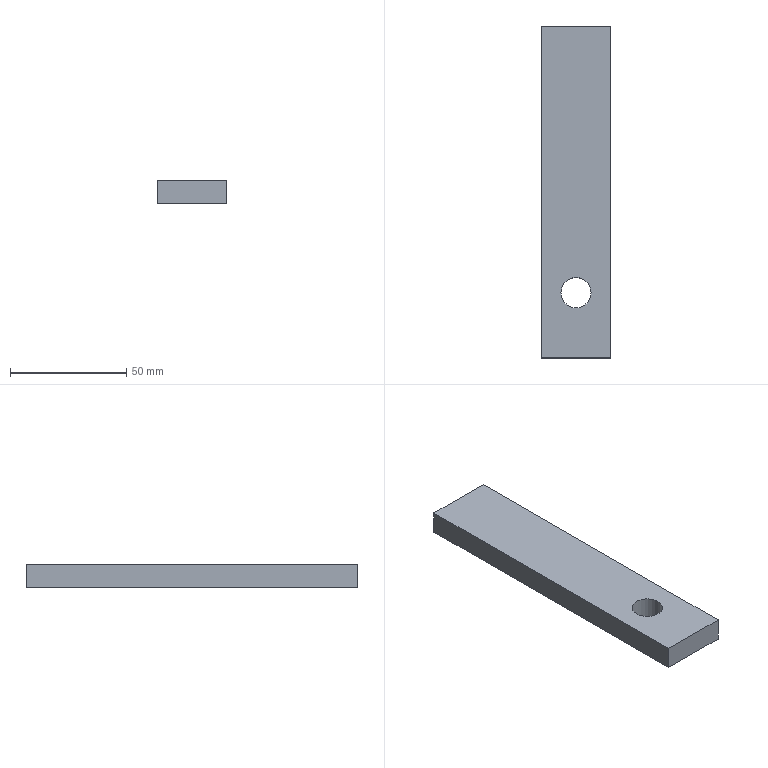Part | NX | features solid 2 | 1 solid | 7 faces | box 30 x 142.5 x 10 mm | volume 41423 mm3 | plane 6 | cylinder 1 | commonest cylinder face diameters 13 x1
STEP:
#1=CARTESIAN_POINT('',(15.,-790.,-10.));
#2=VERTEX_POINT('',#1);
#3=CARTESIAN_POINT('',(-15.,-790.,-10.));
#4=VERTEX_POINT('',#3);
#5=CARTESIAN_POINT('',(-15.,-790.,-10.));
#6=DIRECTION('',(1.,0.,0.));
#7=VECTOR('',#6,1000.);
#8=LINE('',#5,#7);
#9=EDGE_CURVE('',#2,#4,#8,.F.);
#10=ORIENTED_EDGE('',*,*,#9,.F.);
#11=CARTESIAN_POINT('',(15.,-647.5,-10.));
#12=VERTEX_POINT('',#11);
#13=CARTESIAN_POINT('',(15.,-700.,-10.));
#14=DIRECTION('',(0.,-1.,0.));
#15=VECTOR('',#14,1000.);
#16=LINE('',#13,#15);
#17=EDGE_CURVE('',#12,#2,#16,.T.);
#18=ORIENTED_EDGE('',*,*,#17,.F.);
#19=CARTESIAN_POINT('',(-15.,-647.5,-10.));
#20=VERTEX_POINT('',#19);
#21=CARTESIAN_POINT('',(-15.,-647.5,-10.));
#22=DIRECTION('',(-1.,0.,0.));
#23=VECTOR('',#22,1000.);
#24=LINE('',#21,#23);
#25=EDGE_CURVE('',#20,#12,#24,.F.);
#26=ORIENTED_EDGE('',*,*,#25,.F.);
#27=CARTESIAN_POINT('',(-15.,-860.,-10.));
#28=DIRECTION('',(0.,1.,0.));
#29=VECTOR('',#28,1000.);
#30=LINE('',#27,#29);
#31=EDGE_CURVE('',#4,#20,#30,.T.);
#32=ORIENTED_EDGE('',*,*,#31,.F.);
#33=EDGE_LOOP('',(#10,#18,#26,#32));
#34=FACE_BOUND('',#33,.T.);
#35=CARTESIAN_POINT('',(6.5,-762.,-10.));
#36=VERTEX_POINT('',#35);
#37=CARTESIAN_POINT('',(0.,-762.,-10.));
#38=DIRECTION('',(0.,0.,-1.));
#39=DIRECTION('',(1.,0.,0.));
#40=AXIS2_PLACEMENT_3D('',#37,#38,#39);
#41=CIRCLE('',#40,6.5);
#42=EDGE_CURVE('',#36,#36,#41,.F.);
#43=ORIENTED_EDGE('',*,*,#42,.F.);
#44=EDGE_LOOP('',(#43));
#45=FACE_BOUND('',#44,.T.);
#46=CARTESIAN_POINT('',(-15.,-860.,-10.));
#47=DIRECTION('',(0.,0.,-1.));
#48=DIRECTION('',(1.,0.,0.));
#49=AXIS2_PLACEMENT_3D('',#46,#47,#48);
#50=PLANE('',#49);
#51=ADVANCED_FACE('',(#34,#45),#50,.F.);
#52=CARTESIAN_POINT('',(15.,-790.,-20.));
#53=VERTEX_POINT('',#52);
#54=CARTESIAN_POINT('',(-15.,-790.,-20.));
#55=VERTEX_POINT('',#54);
#56=CARTESIAN_POINT('',(-15.,-790.,-20.));
#57=DIRECTION('',(1.,0.,0.));
#58=VECTOR('',#57,1000.);
#59=LINE('',#56,#58);
#60=EDGE_CURVE('',#53,#55,#59,.F.);
#61=ORIENTED_EDGE('',*,*,#60,.T.);
#62=CARTESIAN_POINT('',(-15.,-647.5,-20.));
#63=VERTEX_POINT('',#62);
#64=CARTESIAN_POINT('',(-15.,-860.,-20.));
#65=DIRECTION('',(0.,1.,0.));
#66=VECTOR('',#65,1000.);
#67=LINE('',#64,#66);
#68=EDGE_CURVE('',#55,#63,#67,.T.);
#69=ORIENTED_EDGE('',*,*,#68,.T.);
#70=CARTESIAN_POINT('',(15.,-647.5,-20.));
#71=VERTEX_POINT('',#70);
#72=CARTESIAN_POINT('',(-15.,-647.5,-20.));
#73=DIRECTION('',(-1.,0.,0.));
#74=VECTOR('',#73,1000.);
#75=LINE('',#72,#74);
#76=EDGE_CURVE('',#63,#71,#75,.F.);
#77=ORIENTED_EDGE('',*,*,#76,.T.);
#78=CARTESIAN_POINT('',(15.,-700.,-20.));
#79=DIRECTION('',(0.,-1.,0.));
#80=VECTOR('',#79,1000.);
#81=LINE('',#78,#80);
#82=EDGE_CURVE('',#71,#53,#81,.T.);
#83=ORIENTED_EDGE('',*,*,#82,.T.);
#84=EDGE_LOOP('',(#61,#69,#77,#83));
#85=FACE_BOUND('',#84,.T.);
#86=CARTESIAN_POINT('',(6.5,-762.,-20.));
#87=VERTEX_POINT('',#86);
#88=CARTESIAN_POINT('',(0.,-762.,-20.));
#89=DIRECTION('',(0.,0.,-1.));
#90=DIRECTION('',(1.,0.,0.));
#91=AXIS2_PLACEMENT_3D('',#88,#89,#90);
#92=CIRCLE('',#91,6.5);
#93=EDGE_CURVE('',#87,#87,#92,.F.);
#94=ORIENTED_EDGE('',*,*,#93,.T.);
#95=EDGE_LOOP('',(#94));
#96=FACE_BOUND('',#95,.T.);
#97=CARTESIAN_POINT('',(-15.,-860.,-20.));
#98=DIRECTION('',(0.,0.,-1.));
#99=DIRECTION('',(1.,0.,0.));
#100=AXIS2_PLACEMENT_3D('',#97,#98,#99);
#101=PLANE('',#100);
#102=ADVANCED_FACE('',(#85,#96),#101,.T.);
#103=ORIENTED_EDGE('',*,*,#60,.F.);
#104=CARTESIAN_POINT('',(15.,-790.,-10.));
#105=DIRECTION('',(0.,0.,1.));
#106=VECTOR('',#105,1000.);
#107=LINE('',#104,#106);
#108=EDGE_CURVE('',#2,#53,#107,.F.);
#109=ORIENTED_EDGE('',*,*,#108,.F.);
#110=ORIENTED_EDGE('',*,*,#9,.T.);
#111=CARTESIAN_POINT('',(-15.,-790.,-75.));
#112=DIRECTION('',(0.,0.,1.));
#113=VECTOR('',#112,1000.);
#114=LINE('',#111,#113);
#115=EDGE_CURVE('',#4,#55,#114,.F.);
#116=ORIENTED_EDGE('',*,*,#115,.T.);
#117=EDGE_LOOP('',(#103,#109,#110,#116));
#118=FACE_BOUND('',#117,.T.);
#119=CARTESIAN_POINT('',(28.,-790.,-75.));
#120=DIRECTION('',(0.,1.,0.));
#121=DIRECTION('',(0.,0.,-1.));
#122=AXIS2_PLACEMENT_3D('',#119,#120,#121);
#123=PLANE('',#122);
#124=ADVANCED_FACE('',(#118),#123,.F.);
#125=ORIENTED_EDGE('',*,*,#68,.F.);
#126=ORIENTED_EDGE('',*,*,#115,.F.);
#127=ORIENTED_EDGE('',*,*,#31,.T.);
#128=CARTESIAN_POINT('',(-15.,-647.5,-10.));
#129=DIRECTION('',(0.,0.,1.));
#130=VECTOR('',#129,1000.);
#131=LINE('',#128,#130);
#132=EDGE_CURVE('',#20,#63,#131,.F.);
#133=ORIENTED_EDGE('',*,*,#132,.T.);
#134=EDGE_LOOP('',(#125,#126,#127,#133));
#135=FACE_BOUND('',#134,.T.);
#136=CARTESIAN_POINT('',(-15.,-860.,-10.));
#137=DIRECTION('',(-1.,0.,0.));
#138=DIRECTION('',(0.,0.,-1.));
#139=AXIS2_PLACEMENT_3D('',#136,#137,#138);
#140=PLANE('',#139);
#141=ADVANCED_FACE('',(#135),#140,.T.);
#142=ORIENTED_EDGE('',*,*,#76,.F.);
#143=ORIENTED_EDGE('',*,*,#132,.F.);
#144=ORIENTED_EDGE('',*,*,#25,.T.);
#145=CARTESIAN_POINT('',(15.,-647.5,-10.));
#146=DIRECTION('',(0.,0.,1.));
#147=VECTOR('',#146,1000.);
#148=LINE('',#145,#147);
#149=EDGE_CURVE('',#12,#71,#148,.F.);
#150=ORIENTED_EDGE('',*,*,#149,.T.);
#151=EDGE_LOOP('',(#142,#143,#144,#150));
#152=FACE_BOUND('',#151,.T.);
#153=CARTESIAN_POINT('',(130.,-647.5,-10.));
#154=DIRECTION('',(0.,-1.,0.));
#155=DIRECTION('',(0.,0.,1.));
#156=AXIS2_PLACEMENT_3D('',#153,#154,#155);
#157=PLANE('',#156);
#158=ADVANCED_FACE('',(#152),#157,.F.);
#159=ORIENTED_EDGE('',*,*,#82,.F.);
#160=ORIENTED_EDGE('',*,*,#149,.F.);
#161=ORIENTED_EDGE('',*,*,#17,.T.);
#162=ORIENTED_EDGE('',*,*,#108,.T.);
#163=EDGE_LOOP('',(#159,#160,#161,#162));
#164=FACE_BOUND('',#163,.T.);
#165=CARTESIAN_POINT('',(15.,-700.,-10.));
#166=DIRECTION('',(1.,0.,0.));
#167=DIRECTION('',(0.,0.,1.));
#168=AXIS2_PLACEMENT_3D('',#165,#166,#167);
#169=PLANE('',#168);
#170=ADVANCED_FACE('',(#164),#169,.T.);
#171=ORIENTED_EDGE('',*,*,#93,.F.);
#172=EDGE_LOOP('',(#171));
#173=FACE_BOUND('',#172,.T.);
#174=ORIENTED_EDGE('',*,*,#42,.T.);
#175=EDGE_LOOP('',(#174));
#176=FACE_BOUND('',#175,.T.);
#177=CARTESIAN_POINT('',(0.,-762.,104.));
#178=DIRECTION('',(0.,0.,-1.));
#179=DIRECTION('',(1.,0.,0.));
#180=AXIS2_PLACEMENT_3D('',#177,#178,#179);
#181=CYLINDRICAL_SURFACE('',#180,6.5);
#182=ADVANCED_FACE('',(#173,#176),#181,.F.);
#183=CLOSED_SHELL('',(#51,#102,#124,#141,#158,#170,#182));
#184=MANIFOLD_SOLID_BREP('',#183);
#185=(LENGTH_UNIT()NAMED_UNIT(*)SI_UNIT(.MILLI.,.METRE.));
#186=UNCERTAINTY_MEASURE_WITH_UNIT(LENGTH_MEASURE(0.00001),#185,'','');
#187=(NAMED_UNIT(*)PLANE_ANGLE_UNIT()SI_UNIT($,.RADIAN.));
#188=(NAMED_UNIT(*)SI_UNIT($,.STERADIAN.)SOLID_ANGLE_UNIT());
#189=(GEOMETRIC_REPRESENTATION_CONTEXT(3)GLOBAL_UNCERTAINTY_ASSIGNED_CONTEXT((#186))GLOBAL_UNIT_ASSIGNED_CONTEXT((#185,#187,#188))REPRESENTATION_CONTEXT('',''));
#190=ADVANCED_BREP_SHAPE_REPRESENTATION('',(#184),#189);